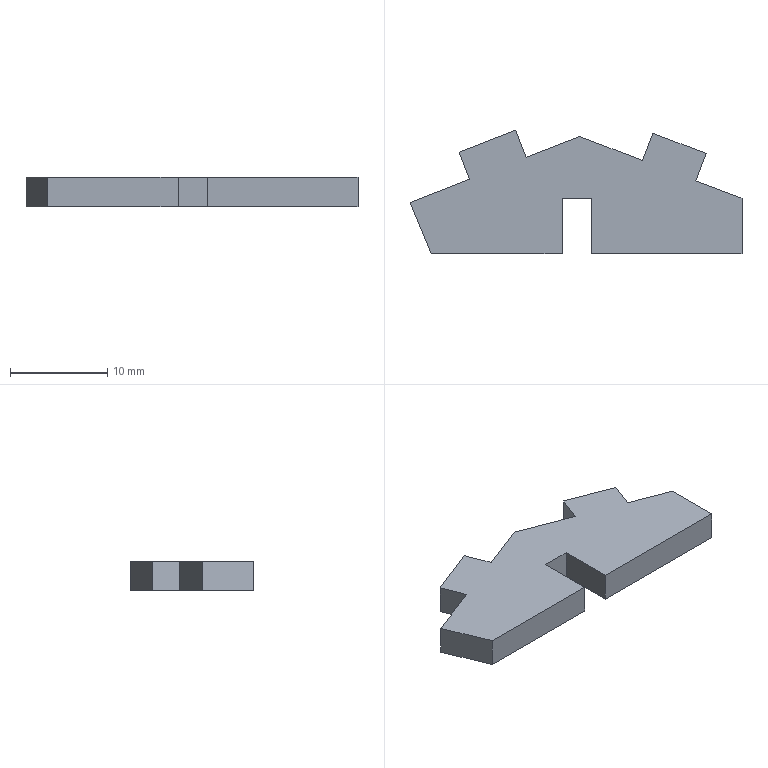Part | SolidWorks | features BaseBody 1 | 1 solid | 19 faces | box 34.167 x 12.73 x 3 mm | volume 940.893 mm3 | plane 19
STEP:
#1=CARTESIAN_POINT('',(0.6585,7.161,-1.5));
#2=VERTEX_POINT('',#1);
#3=CARTESIAN_POINT('',(0.6585,12.877,-1.5));
#4=VERTEX_POINT('',#3);
#5=CARTESIAN_POINT('',(0.6585,7.161,-1.5));
#6=DIRECTION('',(0.,1.,0.));
#7=VECTOR('',#6,1000.);
#8=LINE('',#5,#7);
#9=EDGE_CURVE('',#2,#4,#8,.T.);
#10=ORIENTED_EDGE('',*,*,#9,.F.);
#11=CARTESIAN_POINT('',(-14.855,7.161,-1.5));
#12=VERTEX_POINT('',#11);
#13=CARTESIAN_POINT('',(-14.855,7.161,-1.5));
#14=DIRECTION('',(1.,0.,0.));
#15=VECTOR('',#14,1000.);
#16=LINE('',#13,#15);
#17=EDGE_CURVE('',#12,#2,#16,.T.);
#18=ORIENTED_EDGE('',*,*,#17,.F.);
#19=CARTESIAN_POINT('',(-14.855,12.877,-1.5));
#20=VERTEX_POINT('',#19);
#21=CARTESIAN_POINT('',(-14.855,12.877,-1.5));
#22=DIRECTION('',(0.,-1.,0.));
#23=VECTOR('',#22,1000.);
#24=LINE('',#21,#23);
#25=EDGE_CURVE('',#20,#12,#24,.T.);
#26=ORIENTED_EDGE('',*,*,#25,.F.);
#27=CARTESIAN_POINT('',(-17.852,12.877,-1.5));
#28=VERTEX_POINT('',#27);
#29=CARTESIAN_POINT('',(-17.852,12.877,-1.5));
#30=DIRECTION('',(1.,0.,0.));
#31=VECTOR('',#30,1000.);
#32=LINE('',#29,#31);
#33=EDGE_CURVE('',#28,#20,#32,.T.);
#34=ORIENTED_EDGE('',*,*,#33,.F.);
#35=CARTESIAN_POINT('',(-17.852,7.161,-1.5));
#36=VERTEX_POINT('',#35);
#37=CARTESIAN_POINT('',(-17.852,7.161,-1.5));
#38=DIRECTION('',(0.,1.,0.));
#39=VECTOR('',#38,1000.);
#40=LINE('',#37,#39);
#41=EDGE_CURVE('',#36,#28,#40,.T.);
#42=ORIENTED_EDGE('',*,*,#41,.F.);
#43=CARTESIAN_POINT('',(-31.329,7.161,-1.5));
#44=VERTEX_POINT('',#43);
#45=CARTESIAN_POINT('',(-31.329,7.161,-1.5));
#46=DIRECTION('',(1.,0.,0.));
#47=VECTOR('',#46,1000.);
#48=LINE('',#45,#47);
#49=EDGE_CURVE('',#44,#36,#48,.T.);
#50=ORIENTED_EDGE('',*,*,#49,.F.);
#51=CARTESIAN_POINT('',(-33.508,12.449,-1.5));
#52=VERTEX_POINT('',#51);
#53=CARTESIAN_POINT('',(-33.508,12.449,-1.5));
#54=DIRECTION('',(0.381,-0.9246,0.));
#55=VECTOR('',#54,1000.);
#56=LINE('',#53,#55);
#57=EDGE_CURVE('',#52,#44,#56,.T.);
#58=ORIENTED_EDGE('',*,*,#57,.F.);
#59=CARTESIAN_POINT('',(-27.369,14.843,-1.5));
#60=VERTEX_POINT('',#59);
#61=CARTESIAN_POINT('',(-27.369,14.843,-1.5));
#62=DIRECTION('',(-0.9317,-0.3633,0.));
#63=VECTOR('',#62,1000.);
#64=LINE('',#61,#63);
#65=EDGE_CURVE('',#60,#52,#64,.T.);
#66=ORIENTED_EDGE('',*,*,#65,.F.);
#67=CARTESIAN_POINT('',(-28.452,17.626,-1.5));
#68=VERTEX_POINT('',#67);
#69=CARTESIAN_POINT('',(-28.452,17.626,-1.5));
#70=DIRECTION('',(0.3626,-0.9319,0.));
#71=VECTOR('',#70,1000.);
#72=LINE('',#69,#71);
#73=EDGE_CURVE('',#68,#60,#72,.T.);
#74=ORIENTED_EDGE('',*,*,#73,.F.);
#75=CARTESIAN_POINT('',(-22.633,19.891,-1.5));
#76=VERTEX_POINT('',#75);
#77=CARTESIAN_POINT('',(-22.633,19.891,-1.5));
#78=DIRECTION('',(-0.9319,-0.3626,0.));
#79=VECTOR('',#78,1000.);
#80=LINE('',#77,#79);
#81=EDGE_CURVE('',#76,#68,#80,.T.);
#82=ORIENTED_EDGE('',*,*,#81,.F.);
#83=CARTESIAN_POINT('',(-21.546,17.099,-1.5));
#84=VERTEX_POINT('',#83);
#85=CARTESIAN_POINT('',(-21.546,17.099,-1.5));
#86=DIRECTION('',(-0.3626,0.9319,0.));
#87=VECTOR('',#86,1000.);
#88=LINE('',#85,#87);
#89=EDGE_CURVE('',#84,#76,#88,.T.);
#90=ORIENTED_EDGE('',*,*,#89,.F.);
#91=CARTESIAN_POINT('',(-16.058,19.236,-1.5));
#92=VERTEX_POINT('',#91);
#93=CARTESIAN_POINT('',(-16.058,19.236,-1.5));
#94=DIRECTION('',(-0.9319,-0.3627,0.));
#95=VECTOR('',#94,1000.);
#96=LINE('',#93,#95);
#97=EDGE_CURVE('',#92,#84,#96,.T.);
#98=ORIENTED_EDGE('',*,*,#97,.F.);
#99=CARTESIAN_POINT('',(-9.59,16.776,-1.5));
#100=VERTEX_POINT('',#99);
#101=CARTESIAN_POINT('',(-9.59,16.776,-1.5));
#102=DIRECTION('',(-0.9347,0.3555,0.));
#103=VECTOR('',#102,1000.);
#104=LINE('',#101,#103);
#105=EDGE_CURVE('',#100,#92,#104,.T.);
#106=ORIENTED_EDGE('',*,*,#105,.F.);
#107=CARTESIAN_POINT('',(-8.524,19.577,-1.5));
#108=VERTEX_POINT('',#107);
#109=CARTESIAN_POINT('',(-8.524,19.577,-1.5));
#110=DIRECTION('',(-0.3557,-0.9346,0.));
#111=VECTOR('',#110,1000.);
#112=LINE('',#109,#111);
#113=EDGE_CURVE('',#108,#100,#112,.T.);
#114=ORIENTED_EDGE('',*,*,#113,.F.);
#115=CARTESIAN_POINT('',(-3.025,17.484,-1.5));
#116=VERTEX_POINT('',#115);
#117=CARTESIAN_POINT('',(-3.025,17.484,-1.5));
#118=DIRECTION('',(-0.9346,0.3557,0.));
#119=VECTOR('',#118,1000.);
#120=LINE('',#117,#119);
#121=EDGE_CURVE('',#116,#108,#120,.T.);
#122=ORIENTED_EDGE('',*,*,#121,.F.);
#123=CARTESIAN_POINT('',(-4.091,14.684,-1.5));
#124=VERTEX_POINT('',#123);
#125=CARTESIAN_POINT('',(-4.091,14.684,-1.5));
#126=DIRECTION('',(0.3557,0.9346,0.));
#127=VECTOR('',#126,1000.);
#128=LINE('',#125,#127);
#129=EDGE_CURVE('',#124,#116,#128,.T.);
#130=ORIENTED_EDGE('',*,*,#129,.F.);
#131=CARTESIAN_POINT('',(0.6585,12.877,-1.5));
#132=DIRECTION('',(-0.9347,0.3556,0.));
#133=VECTOR('',#132,1000.);
#134=LINE('',#131,#133);
#135=EDGE_CURVE('',#4,#124,#134,.T.);
#136=ORIENTED_EDGE('',*,*,#135,.F.);
#137=EDGE_LOOP('',(#10,#18,#26,#34,#42,#50,#58,#66,#74,#82,#90,#98,#106,#114,#122,#130,#136));
#138=FACE_OUTER_BOUND('',#137,.T.);
#139=CARTESIAN_POINT('',(0.,0.,-1.5));
#140=DIRECTION('',(0.,0.,-1.));
#141=DIRECTION('',(0.,-1.,0.));
#142=AXIS2_PLACEMENT_3D('',#139,#140,#141);
#143=PLANE('',#142);
#144=ADVANCED_FACE('',(#138),#143,.T.);
#145=CARTESIAN_POINT('',(0.6585,7.161,1.5));
#146=VERTEX_POINT('',#145);
#147=CARTESIAN_POINT('',(0.6585,12.877,1.5));
#148=VERTEX_POINT('',#147);
#149=CARTESIAN_POINT('',(0.6585,7.161,1.5));
#150=DIRECTION('',(0.,1.,0.));
#151=VECTOR('',#150,1000.);
#152=LINE('',#149,#151);
#153=EDGE_CURVE('',#146,#148,#152,.T.);
#154=ORIENTED_EDGE('',*,*,#153,.T.);
#155=CARTESIAN_POINT('',(-4.091,14.684,1.5));
#156=VERTEX_POINT('',#155);
#157=CARTESIAN_POINT('',(0.6585,12.877,1.5));
#158=DIRECTION('',(-0.9347,0.3556,0.));
#159=VECTOR('',#158,1000.);
#160=LINE('',#157,#159);
#161=EDGE_CURVE('',#148,#156,#160,.T.);
#162=ORIENTED_EDGE('',*,*,#161,.T.);
#163=CARTESIAN_POINT('',(-3.025,17.484,1.5));
#164=VERTEX_POINT('',#163);
#165=CARTESIAN_POINT('',(-4.091,14.684,1.5));
#166=DIRECTION('',(0.3557,0.9346,0.));
#167=VECTOR('',#166,1000.);
#168=LINE('',#165,#167);
#169=EDGE_CURVE('',#156,#164,#168,.T.);
#170=ORIENTED_EDGE('',*,*,#169,.T.);
#171=CARTESIAN_POINT('',(-8.524,19.577,1.5));
#172=VERTEX_POINT('',#171);
#173=CARTESIAN_POINT('',(-3.025,17.484,1.5));
#174=DIRECTION('',(-0.9346,0.3557,0.));
#175=VECTOR('',#174,1000.);
#176=LINE('',#173,#175);
#177=EDGE_CURVE('',#164,#172,#176,.T.);
#178=ORIENTED_EDGE('',*,*,#177,.T.);
#179=CARTESIAN_POINT('',(-9.59,16.776,1.5));
#180=VERTEX_POINT('',#179);
#181=CARTESIAN_POINT('',(-8.524,19.577,1.5));
#182=DIRECTION('',(-0.3557,-0.9346,0.));
#183=VECTOR('',#182,1000.);
#184=LINE('',#181,#183);
#185=EDGE_CURVE('',#172,#180,#184,.T.);
#186=ORIENTED_EDGE('',*,*,#185,.T.);
#187=CARTESIAN_POINT('',(-16.058,19.236,1.5));
#188=VERTEX_POINT('',#187);
#189=CARTESIAN_POINT('',(-9.59,16.776,1.5));
#190=DIRECTION('',(-0.9347,0.3555,0.));
#191=VECTOR('',#190,1000.);
#192=LINE('',#189,#191);
#193=EDGE_CURVE('',#180,#188,#192,.T.);
#194=ORIENTED_EDGE('',*,*,#193,.T.);
#195=CARTESIAN_POINT('',(-21.546,17.099,1.5));
#196=VERTEX_POINT('',#195);
#197=CARTESIAN_POINT('',(-16.058,19.236,1.5));
#198=DIRECTION('',(-0.9319,-0.3627,0.));
#199=VECTOR('',#198,1000.);
#200=LINE('',#197,#199);
#201=EDGE_CURVE('',#188,#196,#200,.T.);
#202=ORIENTED_EDGE('',*,*,#201,.T.);
#203=CARTESIAN_POINT('',(-22.633,19.891,1.5));
#204=VERTEX_POINT('',#203);
#205=CARTESIAN_POINT('',(-21.546,17.099,1.5));
#206=DIRECTION('',(-0.3626,0.9319,0.));
#207=VECTOR('',#206,1000.);
#208=LINE('',#205,#207);
#209=EDGE_CURVE('',#196,#204,#208,.T.);
#210=ORIENTED_EDGE('',*,*,#209,.T.);
#211=CARTESIAN_POINT('',(-28.452,17.626,1.5));
#212=VERTEX_POINT('',#211);
#213=CARTESIAN_POINT('',(-22.633,19.891,1.5));
#214=DIRECTION('',(-0.9319,-0.3626,0.));
#215=VECTOR('',#214,1000.);
#216=LINE('',#213,#215);
#217=EDGE_CURVE('',#204,#212,#216,.T.);
#218=ORIENTED_EDGE('',*,*,#217,.T.);
#219=CARTESIAN_POINT('',(-27.369,14.843,1.5));
#220=VERTEX_POINT('',#219);
#221=CARTESIAN_POINT('',(-28.452,17.626,1.5));
#222=DIRECTION('',(0.3626,-0.9319,0.));
#223=VECTOR('',#222,1000.);
#224=LINE('',#221,#223);
#225=EDGE_CURVE('',#212,#220,#224,.T.);
#226=ORIENTED_EDGE('',*,*,#225,.T.);
#227=CARTESIAN_POINT('',(-33.508,12.449,1.5));
#228=VERTEX_POINT('',#227);
#229=CARTESIAN_POINT('',(-27.369,14.843,1.5));
#230=DIRECTION('',(-0.9317,-0.3633,0.));
#231=VECTOR('',#230,1000.);
#232=LINE('',#229,#231);
#233=EDGE_CURVE('',#220,#228,#232,.T.);
#234=ORIENTED_EDGE('',*,*,#233,.T.);
#235=CARTESIAN_POINT('',(-31.329,7.161,1.5));
#236=VERTEX_POINT('',#235);
#237=CARTESIAN_POINT('',(-33.508,12.449,1.5));
#238=DIRECTION('',(0.381,-0.9246,0.));
#239=VECTOR('',#238,1000.);
#240=LINE('',#237,#239);
#241=EDGE_CURVE('',#228,#236,#240,.T.);
#242=ORIENTED_EDGE('',*,*,#241,.T.);
#243=CARTESIAN_POINT('',(-17.852,7.161,1.5));
#244=VERTEX_POINT('',#243);
#245=CARTESIAN_POINT('',(-31.329,7.161,1.5));
#246=DIRECTION('',(1.,0.,0.));
#247=VECTOR('',#246,1000.);
#248=LINE('',#245,#247);
#249=EDGE_CURVE('',#236,#244,#248,.T.);
#250=ORIENTED_EDGE('',*,*,#249,.T.);
#251=CARTESIAN_POINT('',(-17.852,12.877,1.5));
#252=VERTEX_POINT('',#251);
#253=CARTESIAN_POINT('',(-17.852,7.161,1.5));
#254=DIRECTION('',(0.,1.,0.));
#255=VECTOR('',#254,1000.);
#256=LINE('',#253,#255);
#257=EDGE_CURVE('',#244,#252,#256,.T.);
#258=ORIENTED_EDGE('',*,*,#257,.T.);
#259=CARTESIAN_POINT('',(-14.855,12.877,1.5));
#260=VERTEX_POINT('',#259);
#261=CARTESIAN_POINT('',(-17.852,12.877,1.5));
#262=DIRECTION('',(1.,0.,0.));
#263=VECTOR('',#262,1000.);
#264=LINE('',#261,#263);
#265=EDGE_CURVE('',#252,#260,#264,.T.);
#266=ORIENTED_EDGE('',*,*,#265,.T.);
#267=CARTESIAN_POINT('',(-14.855,7.161,1.5));
#268=VERTEX_POINT('',#267);
#269=CARTESIAN_POINT('',(-14.855,12.877,1.5));
#270=DIRECTION('',(0.,-1.,0.));
#271=VECTOR('',#270,1000.);
#272=LINE('',#269,#271);
#273=EDGE_CURVE('',#260,#268,#272,.T.);
#274=ORIENTED_EDGE('',*,*,#273,.T.);
#275=CARTESIAN_POINT('',(-14.855,7.161,1.5));
#276=DIRECTION('',(1.,0.,0.));
#277=VECTOR('',#276,1000.);
#278=LINE('',#275,#277);
#279=EDGE_CURVE('',#268,#146,#278,.T.);
#280=ORIENTED_EDGE('',*,*,#279,.T.);
#281=EDGE_LOOP('',(#154,#162,#170,#178,#186,#194,#202,#210,#218,#226,#234,#242,#250,#258,#266,#274,#280));
#282=FACE_OUTER_BOUND('',#281,.T.);
#283=CARTESIAN_POINT('',(0.,0.,1.5));
#284=DIRECTION('',(0.,0.,-1.));
#285=DIRECTION('',(0.,-1.,0.));
#286=AXIS2_PLACEMENT_3D('',#283,#284,#285);
#287=PLANE('',#286);
#288=ADVANCED_FACE('',(#282),#287,.F.);
#289=ORIENTED_EDGE('',*,*,#17,.T.);
#290=CARTESIAN_POINT('',(0.6585,7.161,1.5));
#291=DIRECTION('',(0.,0.,-1.));
#292=VECTOR('',#291,1000.);
#293=LINE('',#290,#292);
#294=EDGE_CURVE('',#146,#2,#293,.T.);
#295=ORIENTED_EDGE('',*,*,#294,.F.);
#296=ORIENTED_EDGE('',*,*,#279,.F.);
#297=CARTESIAN_POINT('',(-14.855,7.161,1.5));
#298=DIRECTION('',(0.,0.,-1.));
#299=VECTOR('',#298,1000.);
#300=LINE('',#297,#299);
#301=EDGE_CURVE('',#268,#12,#300,.T.);
#302=ORIENTED_EDGE('',*,*,#301,.T.);
#303=EDGE_LOOP('',(#289,#295,#296,#302));
#304=FACE_OUTER_BOUND('',#303,.T.);
#305=CARTESIAN_POINT('',(-14.855,7.161,1.5));
#306=DIRECTION('',(0.,1.,0.));
#307=DIRECTION('',(1.,0.,0.));
#308=AXIS2_PLACEMENT_3D('',#305,#306,#307);
#309=PLANE('',#308);
#310=ADVANCED_FACE('',(#304),#309,.F.);
#311=ORIENTED_EDGE('',*,*,#25,.T.);
#312=ORIENTED_EDGE('',*,*,#301,.F.);
#313=ORIENTED_EDGE('',*,*,#273,.F.);
#314=CARTESIAN_POINT('',(-14.855,12.877,1.5));
#315=DIRECTION('',(0.,0.,-1.));
#316=VECTOR('',#315,1000.);
#317=LINE('',#314,#316);
#318=EDGE_CURVE('',#260,#20,#317,.T.);
#319=ORIENTED_EDGE('',*,*,#318,.T.);
#320=EDGE_LOOP('',(#311,#312,#313,#319));
#321=FACE_OUTER_BOUND('',#320,.T.);
#322=CARTESIAN_POINT('',(-14.855,12.877,1.5));
#323=DIRECTION('',(1.,0.,0.));
#324=DIRECTION('',(0.,1.,0.));
#325=AXIS2_PLACEMENT_3D('',#322,#323,#324);
#326=PLANE('',#325);
#327=ADVANCED_FACE('',(#321),#326,.F.);
#328=ORIENTED_EDGE('',*,*,#33,.T.);
#329=ORIENTED_EDGE('',*,*,#318,.F.);
#330=ORIENTED_EDGE('',*,*,#265,.F.);
#331=CARTESIAN_POINT('',(-17.852,12.877,1.5));
#332=DIRECTION('',(0.,0.,-1.));
#333=VECTOR('',#332,1000.);
#334=LINE('',#331,#333);
#335=EDGE_CURVE('',#252,#28,#334,.T.);
#336=ORIENTED_EDGE('',*,*,#335,.T.);
#337=EDGE_LOOP('',(#328,#329,#330,#336));
#338=FACE_OUTER_BOUND('',#337,.T.);
#339=CARTESIAN_POINT('',(-17.852,12.877,1.5));
#340=DIRECTION('',(0.,1.,0.));
#341=DIRECTION('',(1.,0.,0.));
#342=AXIS2_PLACEMENT_3D('',#339,#340,#341);
#343=PLANE('',#342);
#344=ADVANCED_FACE('',(#338),#343,.F.);
#345=ORIENTED_EDGE('',*,*,#41,.T.);
#346=ORIENTED_EDGE('',*,*,#335,.F.);
#347=ORIENTED_EDGE('',*,*,#257,.F.);
#348=CARTESIAN_POINT('',(-17.852,7.161,1.5));
#349=DIRECTION('',(0.,0.,-1.));
#350=VECTOR('',#349,1000.);
#351=LINE('',#348,#350);
#352=EDGE_CURVE('',#244,#36,#351,.T.);
#353=ORIENTED_EDGE('',*,*,#352,.T.);
#354=EDGE_LOOP('',(#345,#346,#347,#353));
#355=FACE_OUTER_BOUND('',#354,.T.);
#356=CARTESIAN_POINT('',(-17.852,7.161,1.5));
#357=DIRECTION('',(-1.,0.,0.));
#358=DIRECTION('',(0.,0.,1.));
#359=AXIS2_PLACEMENT_3D('',#356,#357,#358);
#360=PLANE('',#359);
#361=ADVANCED_FACE('',(#355),#360,.F.);
#362=ORIENTED_EDGE('',*,*,#49,.T.);
#363=ORIENTED_EDGE('',*,*,#352,.F.);
#364=ORIENTED_EDGE('',*,*,#249,.F.);
#365=CARTESIAN_POINT('',(-31.329,7.161,1.5));
#366=DIRECTION('',(0.,0.,-1.));
#367=VECTOR('',#366,1000.);
#368=LINE('',#365,#367);
#369=EDGE_CURVE('',#236,#44,#368,.T.);
#370=ORIENTED_EDGE('',*,*,#369,.T.);
#371=EDGE_LOOP('',(#362,#363,#364,#370));
#372=FACE_OUTER_BOUND('',#371,.T.);
#373=CARTESIAN_POINT('',(-31.329,7.161,1.5));
#374=DIRECTION('',(0.,1.,0.));
#375=DIRECTION('',(1.,0.,0.));
#376=AXIS2_PLACEMENT_3D('',#373,#374,#375);
#377=PLANE('',#376);
#378=ADVANCED_FACE('',(#372),#377,.F.);
#379=ORIENTED_EDGE('',*,*,#57,.T.);
#380=ORIENTED_EDGE('',*,*,#369,.F.);
#381=ORIENTED_EDGE('',*,*,#241,.F.);
#382=CARTESIAN_POINT('',(-33.508,12.449,1.5));
#383=DIRECTION('',(0.,0.,-1.));
#384=VECTOR('',#383,1000.);
#385=LINE('',#382,#384);
#386=EDGE_CURVE('',#228,#52,#385,.T.);
#387=ORIENTED_EDGE('',*,*,#386,.T.);
#388=EDGE_LOOP('',(#379,#380,#381,#387));
#389=FACE_OUTER_BOUND('',#388,.T.);
#390=CARTESIAN_POINT('',(-33.508,12.449,1.5));
#391=DIRECTION('',(0.9246,0.381,0.));
#392=DIRECTION('',(0.,0.,-1.));
#393=AXIS2_PLACEMENT_3D('',#390,#391,#392);
#394=PLANE('',#393);
#395=ADVANCED_FACE('',(#389),#394,.F.);
#396=ORIENTED_EDGE('',*,*,#65,.T.);
#397=ORIENTED_EDGE('',*,*,#386,.F.);
#398=ORIENTED_EDGE('',*,*,#233,.F.);
#399=CARTESIAN_POINT('',(-27.369,14.843,1.5));
#400=DIRECTION('',(0.,0.,-1.));
#401=VECTOR('',#400,1000.);
#402=LINE('',#399,#401);
#403=EDGE_CURVE('',#220,#60,#402,.T.);
#404=ORIENTED_EDGE('',*,*,#403,.T.);
#405=EDGE_LOOP('',(#396,#397,#398,#404));
#406=FACE_OUTER_BOUND('',#405,.T.);
#407=CARTESIAN_POINT('',(-27.369,14.843,1.5));
#408=DIRECTION('',(0.3633,-0.9317,0.));
#409=DIRECTION('',(0.,0.,-1.));
#410=AXIS2_PLACEMENT_3D('',#407,#408,#409);
#411=PLANE('',#410);
#412=ADVANCED_FACE('',(#406),#411,.F.);
#413=ORIENTED_EDGE('',*,*,#73,.T.);
#414=ORIENTED_EDGE('',*,*,#403,.F.);
#415=ORIENTED_EDGE('',*,*,#225,.F.);
#416=CARTESIAN_POINT('',(-28.452,17.626,1.5));
#417=DIRECTION('',(0.,0.,-1.));
#418=VECTOR('',#417,1000.);
#419=LINE('',#416,#418);
#420=EDGE_CURVE('',#212,#68,#419,.T.);
#421=ORIENTED_EDGE('',*,*,#420,.T.);
#422=EDGE_LOOP('',(#413,#414,#415,#421));
#423=FACE_OUTER_BOUND('',#422,.T.);
#424=CARTESIAN_POINT('',(-28.452,17.626,1.5));
#425=DIRECTION('',(0.9319,0.3626,0.));
#426=DIRECTION('',(0.,0.,-1.));
#427=AXIS2_PLACEMENT_3D('',#424,#425,#426);
#428=PLANE('',#427);
#429=ADVANCED_FACE('',(#423),#428,.F.);
#430=ORIENTED_EDGE('',*,*,#81,.T.);
#431=ORIENTED_EDGE('',*,*,#420,.F.);
#432=ORIENTED_EDGE('',*,*,#217,.F.);
#433=CARTESIAN_POINT('',(-22.633,19.891,1.5));
#434=DIRECTION('',(0.,0.,-1.));
#435=VECTOR('',#434,1000.);
#436=LINE('',#433,#435);
#437=EDGE_CURVE('',#204,#76,#436,.T.);
#438=ORIENTED_EDGE('',*,*,#437,.T.);
#439=EDGE_LOOP('',(#430,#431,#432,#438));
#440=FACE_OUTER_BOUND('',#439,.T.);
#441=CARTESIAN_POINT('',(-22.633,19.891,1.5));
#442=DIRECTION('',(0.3626,-0.9319,0.));
#443=DIRECTION('',(0.,0.,-1.));
#444=AXIS2_PLACEMENT_3D('',#441,#442,#443);
#445=PLANE('',#444);
#446=ADVANCED_FACE('',(#440),#445,.F.);
#447=ORIENTED_EDGE('',*,*,#89,.T.);
#448=ORIENTED_EDGE('',*,*,#437,.F.);
#449=ORIENTED_EDGE('',*,*,#209,.F.);
#450=CARTESIAN_POINT('',(-21.546,17.099,1.5));
#451=DIRECTION('',(0.,0.,-1.));
#452=VECTOR('',#451,1000.);
#453=LINE('',#450,#452);
#454=EDGE_CURVE('',#196,#84,#453,.T.);
#455=ORIENTED_EDGE('',*,*,#454,.T.);
#456=EDGE_LOOP('',(#447,#448,#449,#455));
#457=FACE_OUTER_BOUND('',#456,.T.);
#458=CARTESIAN_POINT('',(-21.546,17.099,1.5));
#459=DIRECTION('',(-0.9319,-0.3626,0.));
#460=DIRECTION('',(-0.3626,0.9319,0.));
#461=AXIS2_PLACEMENT_3D('',#458,#459,#460);
#462=PLANE('',#461);
#463=ADVANCED_FACE('',(#457),#462,.F.);
#464=ORIENTED_EDGE('',*,*,#97,.T.);
#465=ORIENTED_EDGE('',*,*,#454,.F.);
#466=ORIENTED_EDGE('',*,*,#201,.F.);
#467=CARTESIAN_POINT('',(-16.058,19.236,1.5));
#468=DIRECTION('',(0.,0.,-1.));
#469=VECTOR('',#468,1000.);
#470=LINE('',#467,#469);
#471=EDGE_CURVE('',#188,#92,#470,.T.);
#472=ORIENTED_EDGE('',*,*,#471,.T.);
#473=EDGE_LOOP('',(#464,#465,#466,#472));
#474=FACE_OUTER_BOUND('',#473,.T.);
#475=CARTESIAN_POINT('',(-16.058,19.236,1.5));
#476=DIRECTION('',(0.3627,-0.9319,0.));
#477=DIRECTION('',(0.,0.,-1.));
#478=AXIS2_PLACEMENT_3D('',#475,#476,#477);
#479=PLANE('',#478);
#480=ADVANCED_FACE('',(#474),#479,.F.);
#481=ORIENTED_EDGE('',*,*,#105,.T.);
#482=ORIENTED_EDGE('',*,*,#471,.F.);
#483=ORIENTED_EDGE('',*,*,#193,.F.);
#484=CARTESIAN_POINT('',(-9.59,16.776,1.5));
#485=DIRECTION('',(0.,0.,-1.));
#486=VECTOR('',#485,1000.);
#487=LINE('',#484,#486);
#488=EDGE_CURVE('',#180,#100,#487,.T.);
#489=ORIENTED_EDGE('',*,*,#488,.T.);
#490=EDGE_LOOP('',(#481,#482,#483,#489));
#491=FACE_OUTER_BOUND('',#490,.T.);
#492=CARTESIAN_POINT('',(-9.59,16.776,1.5));
#493=DIRECTION('',(-0.3555,-0.9347,0.));
#494=DIRECTION('',(-0.9347,0.3555,0.));
#495=AXIS2_PLACEMENT_3D('',#492,#493,#494);
#496=PLANE('',#495);
#497=ADVANCED_FACE('',(#491),#496,.F.);
#498=ORIENTED_EDGE('',*,*,#113,.T.);
#499=ORIENTED_EDGE('',*,*,#488,.F.);
#500=ORIENTED_EDGE('',*,*,#185,.F.);
#501=CARTESIAN_POINT('',(-8.524,19.577,1.5));
#502=DIRECTION('',(0.,0.,-1.));
#503=VECTOR('',#502,1000.);
#504=LINE('',#501,#503);
#505=EDGE_CURVE('',#172,#108,#504,.T.);
#506=ORIENTED_EDGE('',*,*,#505,.T.);
#507=EDGE_LOOP('',(#498,#499,#500,#506));
#508=FACE_OUTER_BOUND('',#507,.T.);
#509=CARTESIAN_POINT('',(-8.524,19.577,1.5));
#510=DIRECTION('',(0.9346,-0.3557,0.));
#511=DIRECTION('',(0.,0.,-1.));
#512=AXIS2_PLACEMENT_3D('',#509,#510,#511);
#513=PLANE('',#512);
#514=ADVANCED_FACE('',(#508),#513,.F.);
#515=ORIENTED_EDGE('',*,*,#121,.T.);
#516=ORIENTED_EDGE('',*,*,#505,.F.);
#517=ORIENTED_EDGE('',*,*,#177,.F.);
#518=CARTESIAN_POINT('',(-3.025,17.484,1.5));
#519=DIRECTION('',(0.,0.,-1.));
#520=VECTOR('',#519,1000.);
#521=LINE('',#518,#520);
#522=EDGE_CURVE('',#164,#116,#521,.T.);
#523=ORIENTED_EDGE('',*,*,#522,.T.);
#524=EDGE_LOOP('',(#515,#516,#517,#523));
#525=FACE_OUTER_BOUND('',#524,.T.);
#526=CARTESIAN_POINT('',(-3.025,17.484,1.5));
#527=DIRECTION('',(-0.3557,-0.9346,0.));
#528=DIRECTION('',(-0.9346,0.3557,0.));
#529=AXIS2_PLACEMENT_3D('',#526,#527,#528);
#530=PLANE('',#529);
#531=ADVANCED_FACE('',(#525),#530,.F.);
#532=ORIENTED_EDGE('',*,*,#129,.T.);
#533=ORIENTED_EDGE('',*,*,#522,.F.);
#534=ORIENTED_EDGE('',*,*,#169,.F.);
#535=CARTESIAN_POINT('',(-4.091,14.684,1.5));
#536=DIRECTION('',(0.,0.,-1.));
#537=VECTOR('',#536,1000.);
#538=LINE('',#535,#537);
#539=EDGE_CURVE('',#156,#124,#538,.T.);
#540=ORIENTED_EDGE('',*,*,#539,.T.);
#541=EDGE_LOOP('',(#532,#533,#534,#540));
#542=FACE_OUTER_BOUND('',#541,.T.);
#543=CARTESIAN_POINT('',(-4.091,14.684,1.5));
#544=DIRECTION('',(-0.9346,0.3557,0.));
#545=DIRECTION('',(0.,0.,1.));
#546=AXIS2_PLACEMENT_3D('',#543,#544,#545);
#547=PLANE('',#546);
#548=ADVANCED_FACE('',(#542),#547,.F.);
#549=ORIENTED_EDGE('',*,*,#135,.T.);
#550=ORIENTED_EDGE('',*,*,#539,.F.);
#551=ORIENTED_EDGE('',*,*,#161,.F.);
#552=CARTESIAN_POINT('',(0.6585,12.877,1.5));
#553=DIRECTION('',(0.,0.,-1.));
#554=VECTOR('',#553,1000.);
#555=LINE('',#552,#554);
#556=EDGE_CURVE('',#148,#4,#555,.T.);
#557=ORIENTED_EDGE('',*,*,#556,.T.);
#558=EDGE_LOOP('',(#549,#550,#551,#557));
#559=FACE_OUTER_BOUND('',#558,.T.);
#560=CARTESIAN_POINT('',(0.6585,12.877,1.5));
#561=DIRECTION('',(-0.3556,-0.9347,0.));
#562=DIRECTION('',(-0.9347,0.3556,0.));
#563=AXIS2_PLACEMENT_3D('',#560,#561,#562);
#564=PLANE('',#563);
#565=ADVANCED_FACE('',(#559),#564,.F.);
#566=ORIENTED_EDGE('',*,*,#9,.T.);
#567=ORIENTED_EDGE('',*,*,#556,.F.);
#568=ORIENTED_EDGE('',*,*,#153,.F.);
#569=ORIENTED_EDGE('',*,*,#294,.T.);
#570=EDGE_LOOP('',(#566,#567,#568,#569));
#571=FACE_OUTER_BOUND('',#570,.T.);
#572=CARTESIAN_POINT('',(0.6585,7.161,1.5));
#573=DIRECTION('',(-1.,0.,0.));
#574=DIRECTION('',(0.,0.,1.));
#575=AXIS2_PLACEMENT_3D('',#572,#573,#574);
#576=PLANE('',#575);
#577=ADVANCED_FACE('',(#571),#576,.F.);
#578=CLOSED_SHELL('',(#144,#288,#310,#327,#344,#361,#378,#395,#412,#429,#446,#463,#480,#497,#514,#531,#548,#565,#577));
#579=MANIFOLD_SOLID_BREP('',#578);
#580=CARTESIAN_POINT('',(0.,0.,0.));
#581=DIRECTION('',(0.,0.,1.));
#582=DIRECTION('',(1.,0.,0.));
#583=AXIS2_PLACEMENT_3D('',#580,#581,#582);
#584=(LENGTH_UNIT()NAMED_UNIT(*)SI_UNIT(.MILLI.,.METRE.));
#585=UNCERTAINTY_MEASURE_WITH_UNIT(LENGTH_MEASURE(0.00001),#584,'','');
#586=(NAMED_UNIT(*)PLANE_ANGLE_UNIT()SI_UNIT($,.RADIAN.));
#587=(NAMED_UNIT(*)SI_UNIT($,.STERADIAN.)SOLID_ANGLE_UNIT());
#588=(GEOMETRIC_REPRESENTATION_CONTEXT(3)GLOBAL_UNCERTAINTY_ASSIGNED_CONTEXT((#585))GLOBAL_UNIT_ASSIGNED_CONTEXT((#584,#586,#587))REPRESENTATION_CONTEXT('',''));
#589=ADVANCED_BREP_SHAPE_REPRESENTATION('',(#579,#583),#588);